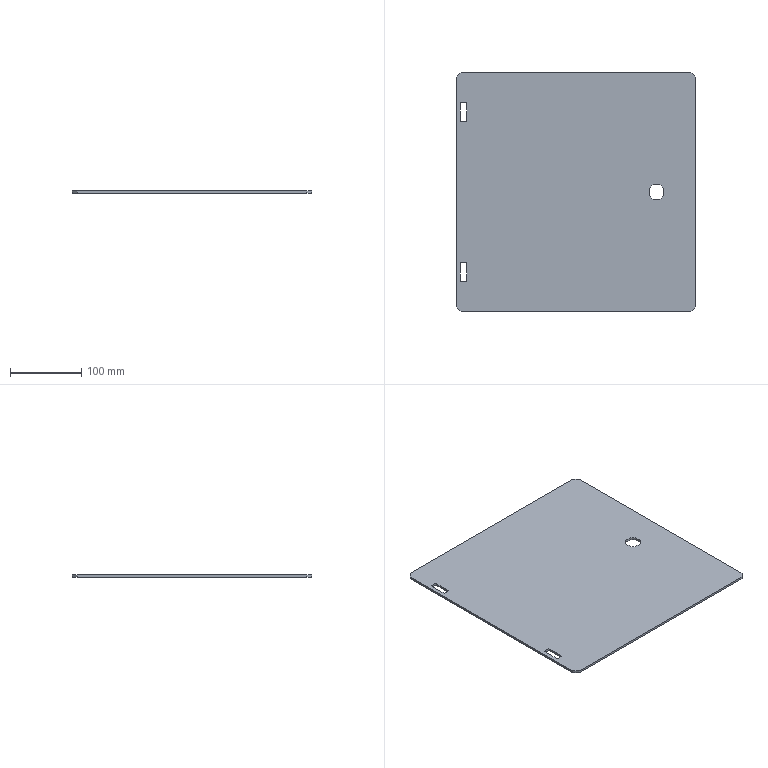Part | SolidWorks | features Extrusion 1, ICE 1 | 1 solid | 26 faces | box 336 x 336 x 3 mm | volume 335960 mm3 | plane 22 | cylinder 4 | commonest cylinder face diameters 22 x4
STEP:
#1=CARTESIAN_POINT('',(-162.2,99.3,3.));
#2=VERTEX_POINT('',#1);
#3=CARTESIAN_POINT('',(-153.2,99.3,3.));
#4=VERTEX_POINT('',#3);
#5=CARTESIAN_POINT('',(-162.2,99.3,3.));
#6=DIRECTION('',(1.,0.,0.));
#7=VECTOR('',#6,1000.);
#8=LINE('',#5,#7);
#9=EDGE_CURVE('',#2,#4,#8,.T.);
#10=ORIENTED_EDGE('',*,*,#9,.F.);
#11=CARTESIAN_POINT('',(-162.2,125.,3.));
#12=VERTEX_POINT('',#11);
#13=CARTESIAN_POINT('',(-162.2,125.,3.));
#14=DIRECTION('',(0.,-1.,0.));
#15=VECTOR('',#14,1000.);
#16=LINE('',#13,#15);
#17=EDGE_CURVE('',#12,#2,#16,.T.);
#18=ORIENTED_EDGE('',*,*,#17,.F.);
#19=CARTESIAN_POINT('',(-153.2,125.,3.));
#20=VERTEX_POINT('',#19);
#21=CARTESIAN_POINT('',(-162.2,125.,3.));
#22=DIRECTION('',(-1.,0.,0.));
#23=VECTOR('',#22,1000.);
#24=LINE('',#21,#23);
#25=EDGE_CURVE('',#20,#12,#24,.T.);
#26=ORIENTED_EDGE('',*,*,#25,.F.);
#27=CARTESIAN_POINT('',(-153.2,125.,3.));
#28=DIRECTION('',(0.,1.,0.));
#29=VECTOR('',#28,1000.);
#30=LINE('',#27,#29);
#31=EDGE_CURVE('',#4,#20,#30,.T.);
#32=ORIENTED_EDGE('',*,*,#31,.F.);
#33=EDGE_LOOP('',(#10,#18,#26,#32));
#34=FACE_BOUND('',#33,.T.);
#35=CARTESIAN_POINT('',(-162.2,-125.,3.));
#36=VERTEX_POINT('',#35);
#37=CARTESIAN_POINT('',(-153.2,-125.,3.));
#38=VERTEX_POINT('',#37);
#39=CARTESIAN_POINT('',(-162.2,-125.,3.));
#40=DIRECTION('',(1.,0.,0.));
#41=VECTOR('',#40,1000.);
#42=LINE('',#39,#41);
#43=EDGE_CURVE('',#36,#38,#42,.T.);
#44=ORIENTED_EDGE('',*,*,#43,.F.);
#45=CARTESIAN_POINT('',(-162.2,-99.3,3.));
#46=VERTEX_POINT('',#45);
#47=CARTESIAN_POINT('',(-162.2,-99.3,3.));
#48=DIRECTION('',(0.,-1.,0.));
#49=VECTOR('',#48,1000.);
#50=LINE('',#47,#49);
#51=EDGE_CURVE('',#46,#36,#50,.T.);
#52=ORIENTED_EDGE('',*,*,#51,.F.);
#53=CARTESIAN_POINT('',(-153.2,-99.3,3.));
#54=VERTEX_POINT('',#53);
#55=CARTESIAN_POINT('',(-162.2,-99.3,3.));
#56=DIRECTION('',(-1.,0.,0.));
#57=VECTOR('',#56,1000.);
#58=LINE('',#55,#57);
#59=EDGE_CURVE('',#54,#46,#58,.T.);
#60=ORIENTED_EDGE('',*,*,#59,.F.);
#61=CARTESIAN_POINT('',(-153.2,-99.3,3.));
#62=DIRECTION('',(0.,1.,0.));
#63=VECTOR('',#62,1000.);
#64=LINE('',#61,#63);
#65=EDGE_CURVE('',#38,#54,#64,.T.);
#66=ORIENTED_EDGE('',*,*,#65,.F.);
#67=EDGE_LOOP('',(#44,#52,#60,#66));
#68=FACE_BOUND('',#67,.T.);
#69=CARTESIAN_POINT('',(103.,4.583,3.));
#70=VERTEX_POINT('',#69);
#71=CARTESIAN_POINT('',(103.,-4.583,3.));
#72=VERTEX_POINT('',#71);
#73=CARTESIAN_POINT('',(103.,4.583,3.));
#74=DIRECTION('',(0.,-1.,0.));
#75=VECTOR('',#74,1000.);
#76=LINE('',#73,#75);
#77=EDGE_CURVE('',#70,#72,#76,.T.);
#78=ORIENTED_EDGE('',*,*,#77,.F.);
#79=CARTESIAN_POINT('',(108.417,10.,3.));
#80=VERTEX_POINT('',#79);
#81=CARTESIAN_POINT('',(113.,0.,3.));
#82=DIRECTION('',(0.,0.,1.));
#83=DIRECTION('',(1.,0.,0.));
#84=AXIS2_PLACEMENT_3D('',#81,#82,#83);
#85=CIRCLE('',#84,11.);
#86=EDGE_CURVE('',#80,#70,#85,.T.);
#87=ORIENTED_EDGE('',*,*,#86,.F.);
#88=CARTESIAN_POINT('',(117.583,10.,3.));
#89=VERTEX_POINT('',#88);
#90=CARTESIAN_POINT('',(108.417,10.,3.));
#91=DIRECTION('',(-1.,0.,0.));
#92=VECTOR('',#91,1000.);
#93=LINE('',#90,#92);
#94=EDGE_CURVE('',#89,#80,#93,.T.);
#95=ORIENTED_EDGE('',*,*,#94,.F.);
#96=CARTESIAN_POINT('',(123.,4.583,3.));
#97=VERTEX_POINT('',#96);
#98=CARTESIAN_POINT('',(113.,0.,3.));
#99=DIRECTION('',(0.,0.,1.));
#100=DIRECTION('',(1.,0.,0.));
#101=AXIS2_PLACEMENT_3D('',#98,#99,#100);
#102=CIRCLE('',#101,11.);
#103=EDGE_CURVE('',#97,#89,#102,.T.);
#104=ORIENTED_EDGE('',*,*,#103,.F.);
#105=CARTESIAN_POINT('',(123.,-4.583,3.));
#106=VERTEX_POINT('',#105);
#107=CARTESIAN_POINT('',(123.,4.583,3.));
#108=DIRECTION('',(0.,1.,0.));
#109=VECTOR('',#108,1000.);
#110=LINE('',#107,#109);
#111=EDGE_CURVE('',#106,#97,#110,.T.);
#112=ORIENTED_EDGE('',*,*,#111,.F.);
#113=CARTESIAN_POINT('',(117.583,-10.,3.));
#114=VERTEX_POINT('',#113);
#115=CARTESIAN_POINT('',(113.,0.,3.));
#116=DIRECTION('',(0.,0.,1.));
#117=DIRECTION('',(1.,0.,0.));
#118=AXIS2_PLACEMENT_3D('',#115,#116,#117);
#119=CIRCLE('',#118,11.);
#120=EDGE_CURVE('',#114,#106,#119,.T.);
#121=ORIENTED_EDGE('',*,*,#120,.F.);
#122=CARTESIAN_POINT('',(108.417,-10.,3.));
#123=VERTEX_POINT('',#122);
#124=CARTESIAN_POINT('',(108.417,-10.,3.));
#125=DIRECTION('',(1.,0.,0.));
#126=VECTOR('',#125,1000.);
#127=LINE('',#124,#126);
#128=EDGE_CURVE('',#123,#114,#127,.T.);
#129=ORIENTED_EDGE('',*,*,#128,.F.);
#130=CARTESIAN_POINT('',(113.,0.,3.));
#131=DIRECTION('',(0.,0.,1.));
#132=DIRECTION('',(1.,0.,0.));
#133=AXIS2_PLACEMENT_3D('',#130,#131,#132);
#134=CIRCLE('',#133,11.);
#135=EDGE_CURVE('',#72,#123,#134,.T.);
#136=ORIENTED_EDGE('',*,*,#135,.F.);
#137=EDGE_LOOP('',(#78,#87,#95,#104,#112,#121,#129,#136));
#138=FACE_BOUND('',#137,.T.);
#139=CARTESIAN_POINT('',(161.243,-168.,3.));
#140=VERTEX_POINT('',#139);
#141=CARTESIAN_POINT('',(168.,-161.243,3.));
#142=VERTEX_POINT('',#141);
#143=CARTESIAN_POINT('',(161.243,-168.,3.));
#144=DIRECTION('',(0.7071,0.7071,0.));
#145=VECTOR('',#144,1000.);
#146=LINE('',#143,#145);
#147=EDGE_CURVE('',#140,#142,#146,.T.);
#148=ORIENTED_EDGE('',*,*,#147,.T.);
#149=CARTESIAN_POINT('',(168.,161.243,3.));
#150=VERTEX_POINT('',#149);
#151=CARTESIAN_POINT('',(168.,-161.243,3.));
#152=DIRECTION('',(0.,1.,0.));
#153=VECTOR('',#152,1000.);
#154=LINE('',#151,#153);
#155=EDGE_CURVE('',#142,#150,#154,.T.);
#156=ORIENTED_EDGE('',*,*,#155,.T.);
#157=CARTESIAN_POINT('',(161.243,168.,3.));
#158=VERTEX_POINT('',#157);
#159=CARTESIAN_POINT('',(168.,161.243,3.));
#160=DIRECTION('',(-0.7071,0.7071,0.));
#161=VECTOR('',#160,1000.);
#162=LINE('',#159,#161);
#163=EDGE_CURVE('',#150,#158,#162,.T.);
#164=ORIENTED_EDGE('',*,*,#163,.T.);
#165=CARTESIAN_POINT('',(-161.243,168.,3.));
#166=VERTEX_POINT('',#165);
#167=CARTESIAN_POINT('',(161.243,168.,3.));
#168=DIRECTION('',(-1.,0.,0.));
#169=VECTOR('',#168,1000.);
#170=LINE('',#167,#169);
#171=EDGE_CURVE('',#158,#166,#170,.T.);
#172=ORIENTED_EDGE('',*,*,#171,.T.);
#173=CARTESIAN_POINT('',(-168.,161.243,3.));
#174=VERTEX_POINT('',#173);
#175=CARTESIAN_POINT('',(-161.243,168.,3.));
#176=DIRECTION('',(-0.7071,-0.7071,0.));
#177=VECTOR('',#176,1000.);
#178=LINE('',#175,#177);
#179=EDGE_CURVE('',#166,#174,#178,.T.);
#180=ORIENTED_EDGE('',*,*,#179,.T.);
#181=CARTESIAN_POINT('',(-168.,-161.243,3.));
#182=VERTEX_POINT('',#181);
#183=CARTESIAN_POINT('',(-168.,161.243,3.));
#184=DIRECTION('',(0.,-1.,0.));
#185=VECTOR('',#184,1000.);
#186=LINE('',#183,#185);
#187=EDGE_CURVE('',#174,#182,#186,.T.);
#188=ORIENTED_EDGE('',*,*,#187,.T.);
#189=CARTESIAN_POINT('',(-161.243,-168.,3.));
#190=VERTEX_POINT('',#189);
#191=CARTESIAN_POINT('',(-168.,-161.243,3.));
#192=DIRECTION('',(0.7071,-0.7071,0.));
#193=VECTOR('',#192,1000.);
#194=LINE('',#191,#193);
#195=EDGE_CURVE('',#182,#190,#194,.T.);
#196=ORIENTED_EDGE('',*,*,#195,.T.);
#197=CARTESIAN_POINT('',(-161.243,-168.,3.));
#198=DIRECTION('',(1.,0.,0.));
#199=VECTOR('',#198,1000.);
#200=LINE('',#197,#199);
#201=EDGE_CURVE('',#190,#140,#200,.T.);
#202=ORIENTED_EDGE('',*,*,#201,.T.);
#203=EDGE_LOOP('',(#148,#156,#164,#172,#180,#188,#196,#202));
#204=FACE_OUTER_BOUND('',#203,.T.);
#205=CARTESIAN_POINT('',(0.,0.,3.));
#206=DIRECTION('',(0.,0.,1.));
#207=DIRECTION('',(1.,0.,0.));
#208=AXIS2_PLACEMENT_3D('',#205,#206,#207);
#209=PLANE('',#208);
#210=ADVANCED_FACE('',(#34,#68,#138,#204),#209,.T.);
#211=CARTESIAN_POINT('',(-162.2,-99.3,0.));
#212=VERTEX_POINT('',#211);
#213=CARTESIAN_POINT('',(-162.2,-125.,0.));
#214=VERTEX_POINT('',#213);
#215=CARTESIAN_POINT('',(-162.2,-99.3,0.));
#216=DIRECTION('',(0.,-1.,0.));
#217=VECTOR('',#216,1000.);
#218=LINE('',#215,#217);
#219=EDGE_CURVE('',#212,#214,#218,.T.);
#220=ORIENTED_EDGE('',*,*,#219,.T.);
#221=CARTESIAN_POINT('',(-153.2,-125.,0.));
#222=VERTEX_POINT('',#221);
#223=CARTESIAN_POINT('',(-162.2,-125.,0.));
#224=DIRECTION('',(1.,0.,0.));
#225=VECTOR('',#224,1000.);
#226=LINE('',#223,#225);
#227=EDGE_CURVE('',#214,#222,#226,.T.);
#228=ORIENTED_EDGE('',*,*,#227,.T.);
#229=CARTESIAN_POINT('',(-153.2,-99.3,0.));
#230=VERTEX_POINT('',#229);
#231=CARTESIAN_POINT('',(-153.2,-99.3,0.));
#232=DIRECTION('',(0.,1.,0.));
#233=VECTOR('',#232,1000.);
#234=LINE('',#231,#233);
#235=EDGE_CURVE('',#222,#230,#234,.T.);
#236=ORIENTED_EDGE('',*,*,#235,.T.);
#237=CARTESIAN_POINT('',(-162.2,-99.3,0.));
#238=DIRECTION('',(-1.,0.,0.));
#239=VECTOR('',#238,1000.);
#240=LINE('',#237,#239);
#241=EDGE_CURVE('',#230,#212,#240,.T.);
#242=ORIENTED_EDGE('',*,*,#241,.T.);
#243=EDGE_LOOP('',(#220,#228,#236,#242));
#244=FACE_BOUND('',#243,.T.);
#245=CARTESIAN_POINT('',(-162.2,125.,0.));
#246=VERTEX_POINT('',#245);
#247=CARTESIAN_POINT('',(-162.2,99.3,0.));
#248=VERTEX_POINT('',#247);
#249=CARTESIAN_POINT('',(-162.2,125.,0.));
#250=DIRECTION('',(0.,-1.,0.));
#251=VECTOR('',#250,1000.);
#252=LINE('',#249,#251);
#253=EDGE_CURVE('',#246,#248,#252,.T.);
#254=ORIENTED_EDGE('',*,*,#253,.T.);
#255=CARTESIAN_POINT('',(-153.2,99.3,0.));
#256=VERTEX_POINT('',#255);
#257=CARTESIAN_POINT('',(-162.2,99.3,0.));
#258=DIRECTION('',(1.,0.,0.));
#259=VECTOR('',#258,1000.);
#260=LINE('',#257,#259);
#261=EDGE_CURVE('',#248,#256,#260,.T.);
#262=ORIENTED_EDGE('',*,*,#261,.T.);
#263=CARTESIAN_POINT('',(-153.2,125.,0.));
#264=VERTEX_POINT('',#263);
#265=CARTESIAN_POINT('',(-153.2,125.,0.));
#266=DIRECTION('',(0.,1.,0.));
#267=VECTOR('',#266,1000.);
#268=LINE('',#265,#267);
#269=EDGE_CURVE('',#256,#264,#268,.T.);
#270=ORIENTED_EDGE('',*,*,#269,.T.);
#271=CARTESIAN_POINT('',(-162.2,125.,0.));
#272=DIRECTION('',(-1.,0.,0.));
#273=VECTOR('',#272,1000.);
#274=LINE('',#271,#273);
#275=EDGE_CURVE('',#264,#246,#274,.T.);
#276=ORIENTED_EDGE('',*,*,#275,.T.);
#277=EDGE_LOOP('',(#254,#262,#270,#276));
#278=FACE_BOUND('',#277,.T.);
#279=CARTESIAN_POINT('',(108.417,10.,0.));
#280=VERTEX_POINT('',#279);
#281=CARTESIAN_POINT('',(103.,4.583,0.));
#282=VERTEX_POINT('',#281);
#283=CARTESIAN_POINT('',(113.,0.,0.));
#284=DIRECTION('',(0.,0.,1.));
#285=DIRECTION('',(1.,0.,0.));
#286=AXIS2_PLACEMENT_3D('',#283,#284,#285);
#287=CIRCLE('',#286,11.);
#288=EDGE_CURVE('',#280,#282,#287,.T.);
#289=ORIENTED_EDGE('',*,*,#288,.T.);
#290=CARTESIAN_POINT('',(103.,-4.583,0.));
#291=VERTEX_POINT('',#290);
#292=CARTESIAN_POINT('',(103.,4.583,0.));
#293=DIRECTION('',(0.,-1.,0.));
#294=VECTOR('',#293,1000.);
#295=LINE('',#292,#294);
#296=EDGE_CURVE('',#282,#291,#295,.T.);
#297=ORIENTED_EDGE('',*,*,#296,.T.);
#298=CARTESIAN_POINT('',(108.417,-10.,0.));
#299=VERTEX_POINT('',#298);
#300=CARTESIAN_POINT('',(113.,0.,0.));
#301=DIRECTION('',(0.,0.,1.));
#302=DIRECTION('',(1.,0.,0.));
#303=AXIS2_PLACEMENT_3D('',#300,#301,#302);
#304=CIRCLE('',#303,11.);
#305=EDGE_CURVE('',#291,#299,#304,.T.);
#306=ORIENTED_EDGE('',*,*,#305,.T.);
#307=CARTESIAN_POINT('',(117.583,-10.,0.));
#308=VERTEX_POINT('',#307);
#309=CARTESIAN_POINT('',(108.417,-10.,0.));
#310=DIRECTION('',(1.,0.,0.));
#311=VECTOR('',#310,1000.);
#312=LINE('',#309,#311);
#313=EDGE_CURVE('',#299,#308,#312,.T.);
#314=ORIENTED_EDGE('',*,*,#313,.T.);
#315=CARTESIAN_POINT('',(123.,-4.583,0.));
#316=VERTEX_POINT('',#315);
#317=CARTESIAN_POINT('',(113.,0.,0.));
#318=DIRECTION('',(0.,0.,1.));
#319=DIRECTION('',(1.,0.,0.));
#320=AXIS2_PLACEMENT_3D('',#317,#318,#319);
#321=CIRCLE('',#320,11.);
#322=EDGE_CURVE('',#308,#316,#321,.T.);
#323=ORIENTED_EDGE('',*,*,#322,.T.);
#324=CARTESIAN_POINT('',(123.,4.583,0.));
#325=VERTEX_POINT('',#324);
#326=CARTESIAN_POINT('',(123.,4.583,0.));
#327=DIRECTION('',(0.,1.,0.));
#328=VECTOR('',#327,1000.);
#329=LINE('',#326,#328);
#330=EDGE_CURVE('',#316,#325,#329,.T.);
#331=ORIENTED_EDGE('',*,*,#330,.T.);
#332=CARTESIAN_POINT('',(117.583,10.,0.));
#333=VERTEX_POINT('',#332);
#334=CARTESIAN_POINT('',(113.,0.,0.));
#335=DIRECTION('',(0.,0.,1.));
#336=DIRECTION('',(1.,0.,0.));
#337=AXIS2_PLACEMENT_3D('',#334,#335,#336);
#338=CIRCLE('',#337,11.);
#339=EDGE_CURVE('',#325,#333,#338,.T.);
#340=ORIENTED_EDGE('',*,*,#339,.T.);
#341=CARTESIAN_POINT('',(108.417,10.,0.));
#342=DIRECTION('',(-1.,0.,0.));
#343=VECTOR('',#342,1000.);
#344=LINE('',#341,#343);
#345=EDGE_CURVE('',#333,#280,#344,.T.);
#346=ORIENTED_EDGE('',*,*,#345,.T.);
#347=EDGE_LOOP('',(#289,#297,#306,#314,#323,#331,#340,#346));
#348=FACE_BOUND('',#347,.T.);
#349=CARTESIAN_POINT('',(161.243,-168.,0.));
#350=VERTEX_POINT('',#349);
#351=CARTESIAN_POINT('',(168.,-161.243,0.));
#352=VERTEX_POINT('',#351);
#353=CARTESIAN_POINT('',(161.243,-168.,0.));
#354=DIRECTION('',(0.7071,0.7071,0.));
#355=VECTOR('',#354,1000.);
#356=LINE('',#353,#355);
#357=EDGE_CURVE('',#350,#352,#356,.T.);
#358=ORIENTED_EDGE('',*,*,#357,.F.);
#359=CARTESIAN_POINT('',(-161.243,-168.,0.));
#360=VERTEX_POINT('',#359);
#361=CARTESIAN_POINT('',(-161.243,-168.,0.));
#362=DIRECTION('',(1.,0.,0.));
#363=VECTOR('',#362,1000.);
#364=LINE('',#361,#363);
#365=EDGE_CURVE('',#360,#350,#364,.T.);
#366=ORIENTED_EDGE('',*,*,#365,.F.);
#367=CARTESIAN_POINT('',(-168.,-161.243,0.));
#368=VERTEX_POINT('',#367);
#369=CARTESIAN_POINT('',(-168.,-161.243,0.));
#370=DIRECTION('',(0.7071,-0.7071,0.));
#371=VECTOR('',#370,1000.);
#372=LINE('',#369,#371);
#373=EDGE_CURVE('',#368,#360,#372,.T.);
#374=ORIENTED_EDGE('',*,*,#373,.F.);
#375=CARTESIAN_POINT('',(-168.,161.243,0.));
#376=VERTEX_POINT('',#375);
#377=CARTESIAN_POINT('',(-168.,161.243,0.));
#378=DIRECTION('',(0.,-1.,0.));
#379=VECTOR('',#378,1000.);
#380=LINE('',#377,#379);
#381=EDGE_CURVE('',#376,#368,#380,.T.);
#382=ORIENTED_EDGE('',*,*,#381,.F.);
#383=CARTESIAN_POINT('',(-161.243,168.,0.));
#384=VERTEX_POINT('',#383);
#385=CARTESIAN_POINT('',(-161.243,168.,0.));
#386=DIRECTION('',(-0.7071,-0.7071,0.));
#387=VECTOR('',#386,1000.);
#388=LINE('',#385,#387);
#389=EDGE_CURVE('',#384,#376,#388,.T.);
#390=ORIENTED_EDGE('',*,*,#389,.F.);
#391=CARTESIAN_POINT('',(161.243,168.,0.));
#392=VERTEX_POINT('',#391);
#393=CARTESIAN_POINT('',(161.243,168.,0.));
#394=DIRECTION('',(-1.,0.,0.));
#395=VECTOR('',#394,1000.);
#396=LINE('',#393,#395);
#397=EDGE_CURVE('',#392,#384,#396,.T.);
#398=ORIENTED_EDGE('',*,*,#397,.F.);
#399=CARTESIAN_POINT('',(168.,161.243,0.));
#400=VERTEX_POINT('',#399);
#401=CARTESIAN_POINT('',(168.,161.243,0.));
#402=DIRECTION('',(-0.7071,0.7071,0.));
#403=VECTOR('',#402,1000.);
#404=LINE('',#401,#403);
#405=EDGE_CURVE('',#400,#392,#404,.T.);
#406=ORIENTED_EDGE('',*,*,#405,.F.);
#407=CARTESIAN_POINT('',(168.,-161.243,0.));
#408=DIRECTION('',(0.,1.,0.));
#409=VECTOR('',#408,1000.);
#410=LINE('',#407,#409);
#411=EDGE_CURVE('',#352,#400,#410,.T.);
#412=ORIENTED_EDGE('',*,*,#411,.F.);
#413=EDGE_LOOP('',(#358,#366,#374,#382,#390,#398,#406,#412));
#414=FACE_OUTER_BOUND('',#413,.T.);
#415=CARTESIAN_POINT('',(0.,0.,0.));
#416=DIRECTION('',(0.,0.,1.));
#417=DIRECTION('',(1.,0.,0.));
#418=AXIS2_PLACEMENT_3D('',#415,#416,#417);
#419=PLANE('',#418);
#420=ADVANCED_FACE('',(#244,#278,#348,#414),#419,.F.);
#421=ORIENTED_EDGE('',*,*,#253,.F.);
#422=CARTESIAN_POINT('',(-162.2,125.,3.));
#423=DIRECTION('',(0.,0.,-1.));
#424=VECTOR('',#423,1000.);
#425=LINE('',#422,#424);
#426=EDGE_CURVE('',#12,#246,#425,.T.);
#427=ORIENTED_EDGE('',*,*,#426,.F.);
#428=ORIENTED_EDGE('',*,*,#17,.T.);
#429=CARTESIAN_POINT('',(-162.2,99.3,3.));
#430=DIRECTION('',(0.,0.,-1.));
#431=VECTOR('',#430,1000.);
#432=LINE('',#429,#431);
#433=EDGE_CURVE('',#2,#248,#432,.T.);
#434=ORIENTED_EDGE('',*,*,#433,.T.);
#435=EDGE_LOOP('',(#421,#427,#428,#434));
#436=FACE_OUTER_BOUND('',#435,.T.);
#437=CARTESIAN_POINT('',(-162.2,125.,3.));
#438=DIRECTION('',(1.,0.,0.));
#439=DIRECTION('',(0.,0.,-1.));
#440=AXIS2_PLACEMENT_3D('',#437,#438,#439);
#441=PLANE('',#440);
#442=ADVANCED_FACE('',(#436),#441,.T.);
#443=ORIENTED_EDGE('',*,*,#261,.F.);
#444=ORIENTED_EDGE('',*,*,#433,.F.);
#445=ORIENTED_EDGE('',*,*,#9,.T.);
#446=CARTESIAN_POINT('',(-153.2,99.3,3.));
#447=DIRECTION('',(0.,0.,-1.));
#448=VECTOR('',#447,1000.);
#449=LINE('',#446,#448);
#450=EDGE_CURVE('',#4,#256,#449,.T.);
#451=ORIENTED_EDGE('',*,*,#450,.T.);
#452=EDGE_LOOP('',(#443,#444,#445,#451));
#453=FACE_OUTER_BOUND('',#452,.T.);
#454=CARTESIAN_POINT('',(-162.2,99.3,3.));
#455=DIRECTION('',(0.,1.,0.));
#456=DIRECTION('',(0.,0.,1.));
#457=AXIS2_PLACEMENT_3D('',#454,#455,#456);
#458=PLANE('',#457);
#459=ADVANCED_FACE('',(#453),#458,.T.);
#460=ORIENTED_EDGE('',*,*,#269,.F.);
#461=ORIENTED_EDGE('',*,*,#450,.F.);
#462=ORIENTED_EDGE('',*,*,#31,.T.);
#463=CARTESIAN_POINT('',(-153.2,125.,3.));
#464=DIRECTION('',(0.,0.,-1.));
#465=VECTOR('',#464,1000.);
#466=LINE('',#463,#465);
#467=EDGE_CURVE('',#20,#264,#466,.T.);
#468=ORIENTED_EDGE('',*,*,#467,.T.);
#469=EDGE_LOOP('',(#460,#461,#462,#468));
#470=FACE_OUTER_BOUND('',#469,.T.);
#471=CARTESIAN_POINT('',(-153.2,125.,3.));
#472=DIRECTION('',(-1.,0.,0.));
#473=DIRECTION('',(0.,0.,1.));
#474=AXIS2_PLACEMENT_3D('',#471,#472,#473);
#475=PLANE('',#474);
#476=ADVANCED_FACE('',(#470),#475,.T.);
#477=ORIENTED_EDGE('',*,*,#275,.F.);
#478=ORIENTED_EDGE('',*,*,#467,.F.);
#479=ORIENTED_EDGE('',*,*,#25,.T.);
#480=ORIENTED_EDGE('',*,*,#426,.T.);
#481=EDGE_LOOP('',(#477,#478,#479,#480));
#482=FACE_OUTER_BOUND('',#481,.T.);
#483=CARTESIAN_POINT('',(-162.2,125.,3.));
#484=DIRECTION('',(0.,-1.,0.));
#485=DIRECTION('',(0.,0.,-1.));
#486=AXIS2_PLACEMENT_3D('',#483,#484,#485);
#487=PLANE('',#486);
#488=ADVANCED_FACE('',(#482),#487,.T.);
#489=ORIENTED_EDGE('',*,*,#219,.F.);
#490=CARTESIAN_POINT('',(-162.2,-99.3,3.));
#491=DIRECTION('',(0.,0.,-1.));
#492=VECTOR('',#491,1000.);
#493=LINE('',#490,#492);
#494=EDGE_CURVE('',#46,#212,#493,.T.);
#495=ORIENTED_EDGE('',*,*,#494,.F.);
#496=ORIENTED_EDGE('',*,*,#51,.T.);
#497=CARTESIAN_POINT('',(-162.2,-125.,3.));
#498=DIRECTION('',(0.,0.,-1.));
#499=VECTOR('',#498,1000.);
#500=LINE('',#497,#499);
#501=EDGE_CURVE('',#36,#214,#500,.T.);
#502=ORIENTED_EDGE('',*,*,#501,.T.);
#503=EDGE_LOOP('',(#489,#495,#496,#502));
#504=FACE_OUTER_BOUND('',#503,.T.);
#505=CARTESIAN_POINT('',(-162.2,-99.3,3.));
#506=DIRECTION('',(1.,0.,0.));
#507=DIRECTION('',(0.,0.,-1.));
#508=AXIS2_PLACEMENT_3D('',#505,#506,#507);
#509=PLANE('',#508);
#510=ADVANCED_FACE('',(#504),#509,.T.);
#511=ORIENTED_EDGE('',*,*,#227,.F.);
#512=ORIENTED_EDGE('',*,*,#501,.F.);
#513=ORIENTED_EDGE('',*,*,#43,.T.);
#514=CARTESIAN_POINT('',(-153.2,-125.,3.));
#515=DIRECTION('',(0.,0.,-1.));
#516=VECTOR('',#515,1000.);
#517=LINE('',#514,#516);
#518=EDGE_CURVE('',#38,#222,#517,.T.);
#519=ORIENTED_EDGE('',*,*,#518,.T.);
#520=EDGE_LOOP('',(#511,#512,#513,#519));
#521=FACE_OUTER_BOUND('',#520,.T.);
#522=CARTESIAN_POINT('',(-162.2,-125.,3.));
#523=DIRECTION('',(0.,1.,0.));
#524=DIRECTION('',(0.,0.,1.));
#525=AXIS2_PLACEMENT_3D('',#522,#523,#524);
#526=PLANE('',#525);
#527=ADVANCED_FACE('',(#521),#526,.T.);
#528=ORIENTED_EDGE('',*,*,#235,.F.);
#529=ORIENTED_EDGE('',*,*,#518,.F.);
#530=ORIENTED_EDGE('',*,*,#65,.T.);
#531=CARTESIAN_POINT('',(-153.2,-99.3,3.));
#532=DIRECTION('',(0.,0.,-1.));
#533=VECTOR('',#532,1000.);
#534=LINE('',#531,#533);
#535=EDGE_CURVE('',#54,#230,#534,.T.);
#536=ORIENTED_EDGE('',*,*,#535,.T.);
#537=EDGE_LOOP('',(#528,#529,#530,#536));
#538=FACE_OUTER_BOUND('',#537,.T.);
#539=CARTESIAN_POINT('',(-153.2,-99.3,3.));
#540=DIRECTION('',(-1.,0.,0.));
#541=DIRECTION('',(0.,0.,1.));
#542=AXIS2_PLACEMENT_3D('',#539,#540,#541);
#543=PLANE('',#542);
#544=ADVANCED_FACE('',(#538),#543,.T.);
#545=ORIENTED_EDGE('',*,*,#241,.F.);
#546=ORIENTED_EDGE('',*,*,#535,.F.);
#547=ORIENTED_EDGE('',*,*,#59,.T.);
#548=ORIENTED_EDGE('',*,*,#494,.T.);
#549=EDGE_LOOP('',(#545,#546,#547,#548));
#550=FACE_OUTER_BOUND('',#549,.T.);
#551=CARTESIAN_POINT('',(-162.2,-99.3,3.));
#552=DIRECTION('',(0.,-1.,0.));
#553=DIRECTION('',(0.,0.,-1.));
#554=AXIS2_PLACEMENT_3D('',#551,#552,#553);
#555=PLANE('',#554);
#556=ADVANCED_FACE('',(#550),#555,.T.);
#557=ORIENTED_EDGE('',*,*,#288,.F.);
#558=CARTESIAN_POINT('',(108.417,10.,3.));
#559=DIRECTION('',(0.,0.,-1.));
#560=VECTOR('',#559,1000.);
#561=LINE('',#558,#560);
#562=EDGE_CURVE('',#80,#280,#561,.T.);
#563=ORIENTED_EDGE('',*,*,#562,.F.);
#564=ORIENTED_EDGE('',*,*,#86,.T.);
#565=CARTESIAN_POINT('',(103.,4.583,3.));
#566=DIRECTION('',(0.,0.,-1.));
#567=VECTOR('',#566,1000.);
#568=LINE('',#565,#567);
#569=EDGE_CURVE('',#70,#282,#568,.T.);
#570=ORIENTED_EDGE('',*,*,#569,.T.);
#571=EDGE_LOOP('',(#557,#563,#564,#570));
#572=FACE_OUTER_BOUND('',#571,.T.);
#573=CARTESIAN_POINT('',(113.,0.,3.));
#574=DIRECTION('',(0.,0.,-1.));
#575=DIRECTION('',(-1.,0.,0.));
#576=AXIS2_PLACEMENT_3D('',#573,#574,#575);
#577=CYLINDRICAL_SURFACE('',#576,11.);
#578=ADVANCED_FACE('',(#572),#577,.F.);
#579=ORIENTED_EDGE('',*,*,#296,.F.);
#580=ORIENTED_EDGE('',*,*,#569,.F.);
#581=ORIENTED_EDGE('',*,*,#77,.T.);
#582=CARTESIAN_POINT('',(103.,-4.583,3.));
#583=DIRECTION('',(0.,0.,-1.));
#584=VECTOR('',#583,1000.);
#585=LINE('',#582,#584);
#586=EDGE_CURVE('',#72,#291,#585,.T.);
#587=ORIENTED_EDGE('',*,*,#586,.T.);
#588=EDGE_LOOP('',(#579,#580,#581,#587));
#589=FACE_OUTER_BOUND('',#588,.T.);
#590=CARTESIAN_POINT('',(103.,4.583,3.));
#591=DIRECTION('',(1.,0.,0.));
#592=DIRECTION('',(0.,1.,0.));
#593=AXIS2_PLACEMENT_3D('',#590,#591,#592);
#594=PLANE('',#593);
#595=ADVANCED_FACE('',(#589),#594,.T.);
#596=ORIENTED_EDGE('',*,*,#305,.F.);
#597=ORIENTED_EDGE('',*,*,#586,.F.);
#598=ORIENTED_EDGE('',*,*,#135,.T.);
#599=CARTESIAN_POINT('',(108.417,-10.,3.));
#600=DIRECTION('',(0.,0.,-1.));
#601=VECTOR('',#600,1000.);
#602=LINE('',#599,#601);
#603=EDGE_CURVE('',#123,#299,#602,.T.);
#604=ORIENTED_EDGE('',*,*,#603,.T.);
#605=EDGE_LOOP('',(#596,#597,#598,#604));
#606=FACE_OUTER_BOUND('',#605,.T.);
#607=CARTESIAN_POINT('',(113.,0.,3.));
#608=DIRECTION('',(0.,0.,-1.));
#609=DIRECTION('',(-1.,0.,0.));
#610=AXIS2_PLACEMENT_3D('',#607,#608,#609);
#611=CYLINDRICAL_SURFACE('',#610,11.);
#612=ADVANCED_FACE('',(#606),#611,.F.);
#613=ORIENTED_EDGE('',*,*,#313,.F.);
#614=ORIENTED_EDGE('',*,*,#603,.F.);
#615=ORIENTED_EDGE('',*,*,#128,.T.);
#616=CARTESIAN_POINT('',(117.583,-10.,3.));
#617=DIRECTION('',(0.,0.,-1.));
#618=VECTOR('',#617,1000.);
#619=LINE('',#616,#618);
#620=EDGE_CURVE('',#114,#308,#619,.T.);
#621=ORIENTED_EDGE('',*,*,#620,.T.);
#622=EDGE_LOOP('',(#613,#614,#615,#621));
#623=FACE_OUTER_BOUND('',#622,.T.);
#624=CARTESIAN_POINT('',(108.417,-10.,3.));
#625=DIRECTION('',(0.,1.,0.));
#626=DIRECTION('',(-1.,0.,0.));
#627=AXIS2_PLACEMENT_3D('',#624,#625,#626);
#628=PLANE('',#627);
#629=ADVANCED_FACE('',(#623),#628,.T.);
#630=ORIENTED_EDGE('',*,*,#322,.F.);
#631=ORIENTED_EDGE('',*,*,#620,.F.);
#632=ORIENTED_EDGE('',*,*,#120,.T.);
#633=CARTESIAN_POINT('',(123.,-4.583,3.));
#634=DIRECTION('',(0.,0.,-1.));
#635=VECTOR('',#634,1000.);
#636=LINE('',#633,#635);
#637=EDGE_CURVE('',#106,#316,#636,.T.);
#638=ORIENTED_EDGE('',*,*,#637,.T.);
#639=EDGE_LOOP('',(#630,#631,#632,#638));
#640=FACE_OUTER_BOUND('',#639,.T.);
#641=CARTESIAN_POINT('',(113.,0.,3.));
#642=DIRECTION('',(0.,0.,-1.));
#643=DIRECTION('',(-1.,0.,0.));
#644=AXIS2_PLACEMENT_3D('',#641,#642,#643);
#645=CYLINDRICAL_SURFACE('',#644,11.);
#646=ADVANCED_FACE('',(#640),#645,.F.);
#647=ORIENTED_EDGE('',*,*,#330,.F.);
#648=ORIENTED_EDGE('',*,*,#637,.F.);
#649=ORIENTED_EDGE('',*,*,#111,.T.);
#650=CARTESIAN_POINT('',(123.,4.583,3.));
#651=DIRECTION('',(0.,0.,-1.));
#652=VECTOR('',#651,1000.);
#653=LINE('',#650,#652);
#654=EDGE_CURVE('',#97,#325,#653,.T.);
#655=ORIENTED_EDGE('',*,*,#654,.T.);
#656=EDGE_LOOP('',(#647,#648,#649,#655));
#657=FACE_OUTER_BOUND('',#656,.T.);
#658=CARTESIAN_POINT('',(123.,4.583,3.));
#659=DIRECTION('',(-1.,0.,0.));
#660=DIRECTION('',(0.,0.,1.));
#661=AXIS2_PLACEMENT_3D('',#658,#659,#660);
#662=PLANE('',#661);
#663=ADVANCED_FACE('',(#657),#662,.T.);
#664=ORIENTED_EDGE('',*,*,#339,.F.);
#665=ORIENTED_EDGE('',*,*,#654,.F.);
#666=ORIENTED_EDGE('',*,*,#103,.T.);
#667=CARTESIAN_POINT('',(117.583,10.,3.));
#668=DIRECTION('',(0.,0.,-1.));
#669=VECTOR('',#668,1000.);
#670=LINE('',#667,#669);
#671=EDGE_CURVE('',#89,#333,#670,.T.);
#672=ORIENTED_EDGE('',*,*,#671,.T.);
#673=EDGE_LOOP('',(#664,#665,#666,#672));
#674=FACE_OUTER_BOUND('',#673,.T.);
#675=CARTESIAN_POINT('',(113.,0.,3.));
#676=DIRECTION('',(0.,0.,-1.));
#677=DIRECTION('',(-1.,0.,0.));
#678=AXIS2_PLACEMENT_3D('',#675,#676,#677);
#679=CYLINDRICAL_SURFACE('',#678,11.);
#680=ADVANCED_FACE('',(#674),#679,.F.);
#681=ORIENTED_EDGE('',*,*,#345,.F.);
#682=ORIENTED_EDGE('',*,*,#671,.F.);
#683=ORIENTED_EDGE('',*,*,#94,.T.);
#684=ORIENTED_EDGE('',*,*,#562,.T.);
#685=EDGE_LOOP('',(#681,#682,#683,#684));
#686=FACE_OUTER_BOUND('',#685,.T.);
#687=CARTESIAN_POINT('',(108.417,10.,3.));
#688=DIRECTION('',(0.,-1.,0.));
#689=DIRECTION('',(0.,0.,-1.));
#690=AXIS2_PLACEMENT_3D('',#687,#688,#689);
#691=PLANE('',#690);
#692=ADVANCED_FACE('',(#686),#691,.T.);
#693=ORIENTED_EDGE('',*,*,#147,.F.);
#694=CARTESIAN_POINT('',(161.243,-168.,0.));
#695=DIRECTION('',(0.,0.,1.));
#696=VECTOR('',#695,1000.);
#697=LINE('',#694,#696);
#698=EDGE_CURVE('',#350,#140,#697,.T.);
#699=ORIENTED_EDGE('',*,*,#698,.F.);
#700=ORIENTED_EDGE('',*,*,#357,.T.);
#701=CARTESIAN_POINT('',(168.,-161.243,0.));
#702=DIRECTION('',(0.,0.,1.));
#703=VECTOR('',#702,1000.);
#704=LINE('',#701,#703);
#705=EDGE_CURVE('',#352,#142,#704,.T.);
#706=ORIENTED_EDGE('',*,*,#705,.T.);
#707=EDGE_LOOP('',(#693,#699,#700,#706));
#708=FACE_OUTER_BOUND('',#707,.T.);
#709=CARTESIAN_POINT('',(161.243,-168.,0.));
#710=DIRECTION('',(0.7071,-0.7071,0.));
#711=DIRECTION('',(0.7071,0.7071,0.));
#712=AXIS2_PLACEMENT_3D('',#709,#710,#711);
#713=PLANE('',#712);
#714=ADVANCED_FACE('',(#708),#713,.T.);
#715=ORIENTED_EDGE('',*,*,#201,.F.);
#716=CARTESIAN_POINT('',(-161.243,-168.,0.));
#717=DIRECTION('',(0.,0.,1.));
#718=VECTOR('',#717,1000.);
#719=LINE('',#716,#718);
#720=EDGE_CURVE('',#360,#190,#719,.T.);
#721=ORIENTED_EDGE('',*,*,#720,.F.);
#722=ORIENTED_EDGE('',*,*,#365,.T.);
#723=ORIENTED_EDGE('',*,*,#698,.T.);
#724=EDGE_LOOP('',(#715,#721,#722,#723));
#725=FACE_OUTER_BOUND('',#724,.T.);
#726=CARTESIAN_POINT('',(-161.243,-168.,0.));
#727=DIRECTION('',(0.,-1.,0.));
#728=DIRECTION('',(0.,0.,-1.));
#729=AXIS2_PLACEMENT_3D('',#726,#727,#728);
#730=PLANE('',#729);
#731=ADVANCED_FACE('',(#725),#730,.T.);
#732=ORIENTED_EDGE('',*,*,#195,.F.);
#733=CARTESIAN_POINT('',(-168.,-161.243,0.));
#734=DIRECTION('',(0.,0.,1.));
#735=VECTOR('',#734,1000.);
#736=LINE('',#733,#735);
#737=EDGE_CURVE('',#368,#182,#736,.T.);
#738=ORIENTED_EDGE('',*,*,#737,.F.);
#739=ORIENTED_EDGE('',*,*,#373,.T.);
#740=ORIENTED_EDGE('',*,*,#720,.T.);
#741=EDGE_LOOP('',(#732,#738,#739,#740));
#742=FACE_OUTER_BOUND('',#741,.T.);
#743=CARTESIAN_POINT('',(-168.,-161.243,0.));
#744=DIRECTION('',(-0.7071,-0.7071,0.));
#745=DIRECTION('',(0.7071,-0.7071,0.));
#746=AXIS2_PLACEMENT_3D('',#743,#744,#745);
#747=PLANE('',#746);
#748=ADVANCED_FACE('',(#742),#747,.T.);
#749=ORIENTED_EDGE('',*,*,#187,.F.);
#750=CARTESIAN_POINT('',(-168.,161.243,0.));
#751=DIRECTION('',(0.,0.,1.));
#752=VECTOR('',#751,1000.);
#753=LINE('',#750,#752);
#754=EDGE_CURVE('',#376,#174,#753,.T.);
#755=ORIENTED_EDGE('',*,*,#754,.F.);
#756=ORIENTED_EDGE('',*,*,#381,.T.);
#757=ORIENTED_EDGE('',*,*,#737,.T.);
#758=EDGE_LOOP('',(#749,#755,#756,#757));
#759=FACE_OUTER_BOUND('',#758,.T.);
#760=CARTESIAN_POINT('',(-168.,161.243,0.));
#761=DIRECTION('',(-1.,0.,0.));
#762=DIRECTION('',(0.,0.,1.));
#763=AXIS2_PLACEMENT_3D('',#760,#761,#762);
#764=PLANE('',#763);
#765=ADVANCED_FACE('',(#759),#764,.T.);
#766=ORIENTED_EDGE('',*,*,#179,.F.);
#767=CARTESIAN_POINT('',(-161.243,168.,0.));
#768=DIRECTION('',(0.,0.,1.));
#769=VECTOR('',#768,1000.);
#770=LINE('',#767,#769);
#771=EDGE_CURVE('',#384,#166,#770,.T.);
#772=ORIENTED_EDGE('',*,*,#771,.F.);
#773=ORIENTED_EDGE('',*,*,#389,.T.);
#774=ORIENTED_EDGE('',*,*,#754,.T.);
#775=EDGE_LOOP('',(#766,#772,#773,#774));
#776=FACE_OUTER_BOUND('',#775,.T.);
#777=CARTESIAN_POINT('',(-161.243,168.,0.));
#778=DIRECTION('',(-0.7071,0.7071,0.));
#779=DIRECTION('',(-0.7071,-0.7071,0.));
#780=AXIS2_PLACEMENT_3D('',#777,#778,#779);
#781=PLANE('',#780);
#782=ADVANCED_FACE('',(#776),#781,.T.);
#783=ORIENTED_EDGE('',*,*,#171,.F.);
#784=CARTESIAN_POINT('',(161.243,168.,0.));
#785=DIRECTION('',(0.,0.,1.));
#786=VECTOR('',#785,1000.);
#787=LINE('',#784,#786);
#788=EDGE_CURVE('',#392,#158,#787,.T.);
#789=ORIENTED_EDGE('',*,*,#788,.F.);
#790=ORIENTED_EDGE('',*,*,#397,.T.);
#791=ORIENTED_EDGE('',*,*,#771,.T.);
#792=EDGE_LOOP('',(#783,#789,#790,#791));
#793=FACE_OUTER_BOUND('',#792,.T.);
#794=CARTESIAN_POINT('',(161.243,168.,0.));
#795=DIRECTION('',(0.,1.,0.));
#796=DIRECTION('',(0.,0.,1.));
#797=AXIS2_PLACEMENT_3D('',#794,#795,#796);
#798=PLANE('',#797);
#799=ADVANCED_FACE('',(#793),#798,.T.);
#800=ORIENTED_EDGE('',*,*,#163,.F.);
#801=CARTESIAN_POINT('',(168.,161.243,0.));
#802=DIRECTION('',(0.,0.,1.));
#803=VECTOR('',#802,1000.);
#804=LINE('',#801,#803);
#805=EDGE_CURVE('',#400,#150,#804,.T.);
#806=ORIENTED_EDGE('',*,*,#805,.F.);
#807=ORIENTED_EDGE('',*,*,#405,.T.);
#808=ORIENTED_EDGE('',*,*,#788,.T.);
#809=EDGE_LOOP('',(#800,#806,#807,#808));
#810=FACE_OUTER_BOUND('',#809,.T.);
#811=CARTESIAN_POINT('',(168.,161.243,0.));
#812=DIRECTION('',(0.7071,0.7071,0.));
#813=DIRECTION('',(-0.7071,0.7071,0.));
#814=AXIS2_PLACEMENT_3D('',#811,#812,#813);
#815=PLANE('',#814);
#816=ADVANCED_FACE('',(#810),#815,.T.);
#817=ORIENTED_EDGE('',*,*,#155,.F.);
#818=ORIENTED_EDGE('',*,*,#705,.F.);
#819=ORIENTED_EDGE('',*,*,#411,.T.);
#820=ORIENTED_EDGE('',*,*,#805,.T.);
#821=EDGE_LOOP('',(#817,#818,#819,#820));
#822=FACE_OUTER_BOUND('',#821,.T.);
#823=CARTESIAN_POINT('',(168.,-161.243,0.));
#824=DIRECTION('',(1.,0.,0.));
#825=DIRECTION('',(0.,0.,-1.));
#826=AXIS2_PLACEMENT_3D('',#823,#824,#825);
#827=PLANE('',#826);
#828=ADVANCED_FACE('',(#822),#827,.T.);
#829=CLOSED_SHELL('',(#210,#420,#442,#459,#476,#488,#510,#527,#544,#556,#578,#595,#612,#629,#646,#663,#680,#692,#714,#731,#748,#765,#782,#799,#816,#828));
#830=MANIFOLD_SOLID_BREP('',#829);
#831=CARTESIAN_POINT('',(0.,0.,0.));
#832=DIRECTION('',(0.,0.,1.));
#833=DIRECTION('',(1.,0.,0.));
#834=AXIS2_PLACEMENT_3D('',#831,#832,#833);
#835=(LENGTH_UNIT()NAMED_UNIT(*)SI_UNIT(.MILLI.,.METRE.));
#836=UNCERTAINTY_MEASURE_WITH_UNIT(LENGTH_MEASURE(0.00001),#835,'','');
#837=(NAMED_UNIT(*)PLANE_ANGLE_UNIT()SI_UNIT($,.RADIAN.));
#838=(NAMED_UNIT(*)SI_UNIT($,.STERADIAN.)SOLID_ANGLE_UNIT());
#839=(GEOMETRIC_REPRESENTATION_CONTEXT(3)GLOBAL_UNCERTAINTY_ASSIGNED_CONTEXT((#836))GLOBAL_UNIT_ASSIGNED_CONTEXT((#835,#837,#838))REPRESENTATION_CONTEXT('',''));
#840=ADVANCED_BREP_SHAPE_REPRESENTATION('',(#830,#834),#839);